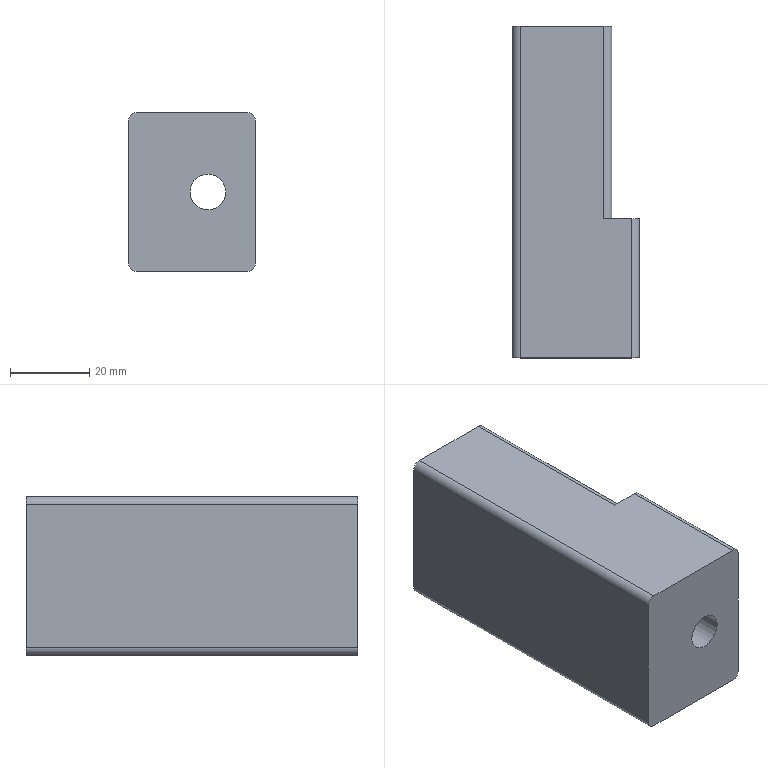Part | Mastercam | 1 solid | 26 faces | box 32 x 83.5 x 40 mm | volume 77489 mm3 | cylinder 15 | plane 11 | commonest cylinder face diameters 4 x8 9 x2 12 x2 16 x2 20 x1
STEP:
#1=CARTESIAN_POINT('',(0.,0.,0.));
#2=DIRECTION('',(0.,0.,1.));
#3=DIRECTION('',(1.,0.,0.));
#4=AXIS2_PLACEMENT_3D('',#1,#2,#3);
#5=CARTESIAN_POINT('',(12.,0.,18.));
#6=VERTEX_POINT('',#5);
#7=CARTESIAN_POINT('',(12.,0.,-18.));
#8=VERTEX_POINT('',#7);
#9=CARTESIAN_POINT('',(12.,0.,18.));
#10=DIRECTION('',(0.,0.,-1.));
#11=VECTOR('',#10,1.);
#12=LINE('',#9,#11);
#13=EDGE_CURVE('',#6,#8,#12,.T.);
#14=ORIENTED_EDGE('',*,*,#13,.F.);
#15=CARTESIAN_POINT('',(10.,0.,20.));
#16=VERTEX_POINT('',#15);
#17=CARTESIAN_POINT('',(10.,0.,18.));
#18=DIRECTION('',(0.,-1.,0.));
#19=DIRECTION('',(1.,0.,0.));
#20=AXIS2_PLACEMENT_3D('',#17,#18,#19);
#21=CIRCLE('',#20,2.);
#22=EDGE_CURVE('',#6,#16,#21,.T.);
#23=ORIENTED_EDGE('',*,*,#22,.T.);
#24=CARTESIAN_POINT('',(-18.,0.,20.));
#25=VERTEX_POINT('',#24);
#26=CARTESIAN_POINT('',(-18.,0.,20.));
#27=DIRECTION('',(1.,0.,0.));
#28=VECTOR('',#27,1.);
#29=LINE('',#26,#28);
#30=EDGE_CURVE('',#25,#16,#29,.T.);
#31=ORIENTED_EDGE('',*,*,#30,.F.);
#32=CARTESIAN_POINT('',(-20.,0.,18.));
#33=VERTEX_POINT('',#32);
#34=CARTESIAN_POINT('',(-18.,0.,18.));
#35=DIRECTION('',(0.,-1.,0.));
#36=DIRECTION('',(0.,0.,1.));
#37=AXIS2_PLACEMENT_3D('',#34,#35,#36);
#38=CIRCLE('',#37,2.);
#39=EDGE_CURVE('',#25,#33,#38,.T.);
#40=ORIENTED_EDGE('',*,*,#39,.T.);
#41=CARTESIAN_POINT('',(-20.,0.,-18.));
#42=VERTEX_POINT('',#41);
#43=CARTESIAN_POINT('',(-20.,0.,-18.));
#44=DIRECTION('',(0.,0.,1.));
#45=VECTOR('',#44,1.);
#46=LINE('',#43,#45);
#47=EDGE_CURVE('',#42,#33,#46,.T.);
#48=ORIENTED_EDGE('',*,*,#47,.F.);
#49=CARTESIAN_POINT('',(-18.,0.,-20.));
#50=VERTEX_POINT('',#49);
#51=CARTESIAN_POINT('',(-18.,0.,-18.));
#52=DIRECTION('',(0.,-1.,0.));
#53=DIRECTION('',(-1.,0.,0.));
#54=AXIS2_PLACEMENT_3D('',#51,#52,#53);
#55=CIRCLE('',#54,2.);
#56=EDGE_CURVE('',#42,#50,#55,.T.);
#57=ORIENTED_EDGE('',*,*,#56,.T.);
#58=CARTESIAN_POINT('',(10.,0.,-20.));
#59=VERTEX_POINT('',#58);
#60=CARTESIAN_POINT('',(10.,0.,-20.));
#61=DIRECTION('',(-1.,0.,0.));
#62=VECTOR('',#61,1.);
#63=LINE('',#60,#62);
#64=EDGE_CURVE('',#59,#50,#63,.T.);
#65=ORIENTED_EDGE('',*,*,#64,.F.);
#66=CARTESIAN_POINT('',(10.,0.,-18.));
#67=DIRECTION('',(0.,-1.,0.));
#68=DIRECTION('',(0.,0.,-1.));
#69=AXIS2_PLACEMENT_3D('',#66,#67,#68);
#70=CIRCLE('',#69,2.);
#71=EDGE_CURVE('',#59,#8,#70,.T.);
#72=ORIENTED_EDGE('',*,*,#71,.T.);
#73=EDGE_LOOP('',(#14,#23,#31,#40,#48,#57,#65,#72));
#74=FACE_OUTER_BOUND('',#73,.T.);
#75=CARTESIAN_POINT('',(4.5,0.,0.));
#76=VERTEX_POINT('',#75);
#77=CARTESIAN_POINT('',(0.,0.,4.5));
#78=VERTEX_POINT('',#77);
#79=CARTESIAN_POINT('',(0.,0.,0.));
#80=DIRECTION('',(0.,-1.,0.));
#81=DIRECTION('',(0.,0.,1.));
#82=AXIS2_PLACEMENT_3D('',#79,#80,#81);
#83=CIRCLE('',#82,4.5);
#84=EDGE_CURVE('',#76,#78,#83,.T.);
#85=ORIENTED_EDGE('',*,*,#84,.F.);
#86=CARTESIAN_POINT('',(-4.5,0.,0.));
#87=VERTEX_POINT('',#86);
#88=CARTESIAN_POINT('',(0.,0.,0.));
#89=DIRECTION('',(0.,-1.,0.));
#90=DIRECTION('',(0.,0.,1.));
#91=AXIS2_PLACEMENT_3D('',#88,#89,#90);
#92=CIRCLE('',#91,4.5);
#93=EDGE_CURVE('',#87,#76,#92,.T.);
#94=ORIENTED_EDGE('',*,*,#93,.F.);
#95=CARTESIAN_POINT('',(0.,0.,0.));
#96=DIRECTION('',(0.,-1.,0.));
#97=DIRECTION('',(0.,0.,1.));
#98=AXIS2_PLACEMENT_3D('',#95,#96,#97);
#99=CIRCLE('',#98,4.5);
#100=EDGE_CURVE('',#78,#87,#99,.T.);
#101=ORIENTED_EDGE('',*,*,#100,.F.);
#102=EDGE_LOOP('',(#85,#94,#101));
#103=FACE_BOUND('',#102,.T.);
#104=CARTESIAN_POINT('',(0.,0.,0.));
#105=DIRECTION('',(0.,1.,0.));
#106=DIRECTION('',(1.,0.,0.));
#107=AXIS2_PLACEMENT_3D('',#104,#105,#106);
#108=PLANE('',#107);
#109=ADVANCED_FACE('',(#74,#103),#108,.F.);
#110=CARTESIAN_POINT('',(-4.5,30.,0.));
#111=VERTEX_POINT('',#110);
#112=CARTESIAN_POINT('',(-4.5,30.,0.));
#113=DIRECTION('',(0.,-1.,0.));
#114=VECTOR('',#113,1.);
#115=LINE('',#112,#114);
#116=EDGE_CURVE('',#111,#87,#115,.T.);
#117=ORIENTED_EDGE('',*,*,#116,.T.);
#118=ORIENTED_EDGE('',*,*,#93,.T.);
#119=CARTESIAN_POINT('',(4.5,30.,0.));
#120=VERTEX_POINT('',#119);
#121=CARTESIAN_POINT('',(4.5,30.,0.));
#122=DIRECTION('',(0.,-1.,0.));
#123=VECTOR('',#122,1.);
#124=LINE('',#121,#123);
#125=EDGE_CURVE('',#120,#76,#124,.T.);
#126=ORIENTED_EDGE('',*,*,#125,.F.);
#127=CARTESIAN_POINT('',(0.,30.,0.));
#128=DIRECTION('',(0.,-1.,0.));
#129=DIRECTION('',(0.,0.,1.));
#130=AXIS2_PLACEMENT_3D('',#127,#128,#129);
#131=CIRCLE('',#130,4.5);
#132=EDGE_CURVE('',#111,#120,#131,.T.);
#133=ORIENTED_EDGE('',*,*,#132,.F.);
#134=EDGE_LOOP('',(#117,#118,#126,#133));
#135=FACE_OUTER_BOUND('',#134,.T.);
#136=CARTESIAN_POINT('',(0.,36.75,0.));
#137=DIRECTION('',(0.,-1.,0.));
#138=DIRECTION('',(0.,0.,1.));
#139=AXIS2_PLACEMENT_3D('',#136,#137,#138);
#140=CYLINDRICAL_SURFACE('',#139,4.5);
#141=ADVANCED_FACE('',(#135),#140,.F.);
#142=CARTESIAN_POINT('',(6.,30.,0.));
#143=VERTEX_POINT('',#142);
#144=CARTESIAN_POINT('',(0.,30.,6.));
#145=VERTEX_POINT('',#144);
#146=CARTESIAN_POINT('',(0.,30.,0.));
#147=DIRECTION('',(0.,-1.,0.));
#148=DIRECTION('',(0.,0.,1.));
#149=AXIS2_PLACEMENT_3D('',#146,#147,#148);
#150=CIRCLE('',#149,6.);
#151=EDGE_CURVE('',#143,#145,#150,.T.);
#152=ORIENTED_EDGE('',*,*,#151,.F.);
#153=CARTESIAN_POINT('',(-6.,30.,0.));
#154=VERTEX_POINT('',#153);
#155=CARTESIAN_POINT('',(0.,30.,0.));
#156=DIRECTION('',(0.,-1.,0.));
#157=DIRECTION('',(0.,0.,1.));
#158=AXIS2_PLACEMENT_3D('',#155,#156,#157);
#159=CIRCLE('',#158,6.);
#160=EDGE_CURVE('',#154,#143,#159,.T.);
#161=ORIENTED_EDGE('',*,*,#160,.F.);
#162=CARTESIAN_POINT('',(0.,30.,0.));
#163=DIRECTION('',(0.,-1.,0.));
#164=DIRECTION('',(0.,0.,1.));
#165=AXIS2_PLACEMENT_3D('',#162,#163,#164);
#166=CIRCLE('',#165,6.);
#167=EDGE_CURVE('',#145,#154,#166,.T.);
#168=ORIENTED_EDGE('',*,*,#167,.F.);
#169=EDGE_LOOP('',(#152,#161,#168));
#170=FACE_OUTER_BOUND('',#169,.T.);
#171=CARTESIAN_POINT('',(0.,30.,4.5));
#172=VERTEX_POINT('',#171);
#173=CARTESIAN_POINT('',(0.,30.,0.));
#174=DIRECTION('',(0.,-1.,0.));
#175=DIRECTION('',(0.,0.,1.));
#176=AXIS2_PLACEMENT_3D('',#173,#174,#175);
#177=CIRCLE('',#176,4.5);
#178=EDGE_CURVE('',#172,#111,#177,.T.);
#179=ORIENTED_EDGE('',*,*,#178,.T.);
#180=ORIENTED_EDGE('',*,*,#132,.T.);
#181=CARTESIAN_POINT('',(0.,30.,0.));
#182=DIRECTION('',(0.,-1.,0.));
#183=DIRECTION('',(0.,0.,1.));
#184=AXIS2_PLACEMENT_3D('',#181,#182,#183);
#185=CIRCLE('',#184,4.5);
#186=EDGE_CURVE('',#120,#172,#185,.T.);
#187=ORIENTED_EDGE('',*,*,#186,.T.);
#188=EDGE_LOOP('',(#179,#180,#187));
#189=FACE_BOUND('',#188,.T.);
#190=CARTESIAN_POINT('',(0.,30.,0.));
#191=DIRECTION('',(0.,-1.,0.));
#192=DIRECTION('',(0.,0.,1.));
#193=AXIS2_PLACEMENT_3D('',#190,#191,#192);
#194=PLANE('',#193);
#195=ADVANCED_FACE('',(#170,#189),#194,.F.);
#196=CARTESIAN_POINT('',(-6.,28.,0.));
#197=VERTEX_POINT('',#196);
#198=CARTESIAN_POINT('',(-6.,30.,0.));
#199=DIRECTION('',(0.,-1.,0.));
#200=VECTOR('',#199,1.);
#201=LINE('',#198,#200);
#202=EDGE_CURVE('',#154,#197,#201,.T.);
#203=ORIENTED_EDGE('',*,*,#202,.F.);
#204=ORIENTED_EDGE('',*,*,#160,.T.);
#205=CARTESIAN_POINT('',(6.,28.,0.));
#206=VERTEX_POINT('',#205);
#207=CARTESIAN_POINT('',(6.,30.,0.));
#208=DIRECTION('',(0.,-1.,0.));
#209=VECTOR('',#208,1.);
#210=LINE('',#207,#209);
#211=EDGE_CURVE('',#143,#206,#210,.T.);
#212=ORIENTED_EDGE('',*,*,#211,.T.);
#213=CARTESIAN_POINT('',(0.,28.,0.));
#214=DIRECTION('',(0.,-1.,0.));
#215=DIRECTION('',(0.,0.,1.));
#216=AXIS2_PLACEMENT_3D('',#213,#214,#215);
#217=CIRCLE('',#216,6.);
#218=EDGE_CURVE('',#197,#206,#217,.T.);
#219=ORIENTED_EDGE('',*,*,#218,.F.);
#220=EDGE_LOOP('',(#203,#204,#212,#219));
#221=FACE_OUTER_BOUND('',#220,.T.);
#222=CARTESIAN_POINT('',(0.,30.1,0.));
#223=DIRECTION('',(0.,-1.,0.));
#224=DIRECTION('',(0.,0.,1.));
#225=AXIS2_PLACEMENT_3D('',#222,#223,#224);
#226=CYLINDRICAL_SURFACE('',#225,6.);
#227=ADVANCED_FACE('',(#221),#226,.T.);
#228=CARTESIAN_POINT('',(8.,28.,0.));
#229=VERTEX_POINT('',#228);
#230=CARTESIAN_POINT('',(0.,28.,8.));
#231=VERTEX_POINT('',#230);
#232=CARTESIAN_POINT('',(0.,28.,0.));
#233=DIRECTION('',(0.,-1.,0.));
#234=DIRECTION('',(0.,0.,1.));
#235=AXIS2_PLACEMENT_3D('',#232,#233,#234);
#236=CIRCLE('',#235,8.);
#237=EDGE_CURVE('',#229,#231,#236,.T.);
#238=ORIENTED_EDGE('',*,*,#237,.F.);
#239=CARTESIAN_POINT('',(-8.,28.,0.));
#240=VERTEX_POINT('',#239);
#241=CARTESIAN_POINT('',(0.,28.,0.));
#242=DIRECTION('',(0.,-1.,0.));
#243=DIRECTION('',(0.,0.,1.));
#244=AXIS2_PLACEMENT_3D('',#241,#242,#243);
#245=CIRCLE('',#244,8.);
#246=EDGE_CURVE('',#240,#229,#245,.T.);
#247=ORIENTED_EDGE('',*,*,#246,.F.);
#248=CARTESIAN_POINT('',(0.,28.,0.));
#249=DIRECTION('',(0.,-1.,0.));
#250=DIRECTION('',(0.,0.,1.));
#251=AXIS2_PLACEMENT_3D('',#248,#249,#250);
#252=CIRCLE('',#251,8.);
#253=EDGE_CURVE('',#231,#240,#252,.T.);
#254=ORIENTED_EDGE('',*,*,#253,.F.);
#255=EDGE_LOOP('',(#238,#247,#254));
#256=FACE_OUTER_BOUND('',#255,.T.);
#257=CARTESIAN_POINT('',(0.,28.,6.));
#258=VERTEX_POINT('',#257);
#259=CARTESIAN_POINT('',(0.,28.,0.));
#260=DIRECTION('',(0.,-1.,0.));
#261=DIRECTION('',(0.,0.,1.));
#262=AXIS2_PLACEMENT_3D('',#259,#260,#261);
#263=CIRCLE('',#262,6.);
#264=EDGE_CURVE('',#258,#197,#263,.T.);
#265=ORIENTED_EDGE('',*,*,#264,.T.);
#266=ORIENTED_EDGE('',*,*,#218,.T.);
#267=CARTESIAN_POINT('',(0.,28.,0.));
#268=DIRECTION('',(0.,-1.,0.));
#269=DIRECTION('',(0.,0.,1.));
#270=AXIS2_PLACEMENT_3D('',#267,#268,#269);
#271=CIRCLE('',#270,6.);
#272=EDGE_CURVE('',#206,#258,#271,.T.);
#273=ORIENTED_EDGE('',*,*,#272,.T.);
#274=EDGE_LOOP('',(#265,#266,#273));
#275=FACE_BOUND('',#274,.T.);
#276=CARTESIAN_POINT('',(0.,28.,0.));
#277=DIRECTION('',(0.,-1.,0.));
#278=DIRECTION('',(0.,0.,1.));
#279=AXIS2_PLACEMENT_3D('',#276,#277,#278);
#280=PLANE('',#279);
#281=ADVANCED_FACE('',(#256,#275),#280,.F.);
#282=CARTESIAN_POINT('',(-8.,35.,0.));
#283=VERTEX_POINT('',#282);
#284=CARTESIAN_POINT('',(-8.,35.,0.));
#285=DIRECTION('',(0.,-1.,0.));
#286=VECTOR('',#285,1.);
#287=LINE('',#284,#286);
#288=EDGE_CURVE('',#283,#240,#287,.T.);
#289=ORIENTED_EDGE('',*,*,#288,.T.);
#290=ORIENTED_EDGE('',*,*,#246,.T.);
#291=CARTESIAN_POINT('',(8.,35.,0.));
#292=VERTEX_POINT('',#291);
#293=CARTESIAN_POINT('',(8.,35.,0.));
#294=DIRECTION('',(0.,-1.,0.));
#295=VECTOR('',#294,1.);
#296=LINE('',#293,#295);
#297=EDGE_CURVE('',#292,#229,#296,.T.);
#298=ORIENTED_EDGE('',*,*,#297,.F.);
#299=CARTESIAN_POINT('',(0.,35.,0.));
#300=DIRECTION('',(0.,-1.,0.));
#301=DIRECTION('',(0.,0.,1.));
#302=AXIS2_PLACEMENT_3D('',#299,#300,#301);
#303=CIRCLE('',#302,8.);
#304=EDGE_CURVE('',#283,#292,#303,.T.);
#305=ORIENTED_EDGE('',*,*,#304,.F.);
#306=EDGE_LOOP('',(#289,#290,#298,#305));
#307=FACE_OUTER_BOUND('',#306,.T.);
#308=CARTESIAN_POINT('',(0.,35.25,0.));
#309=DIRECTION('',(0.,-1.,0.));
#310=DIRECTION('',(0.,0.,1.));
#311=AXIS2_PLACEMENT_3D('',#308,#309,#310);
#312=CYLINDRICAL_SURFACE('',#311,8.);
#313=ADVANCED_FACE('',(#307),#312,.F.);
#314=CARTESIAN_POINT('',(5.,35.,-11.619));
#315=VERTEX_POINT('',#314);
#316=CARTESIAN_POINT('',(2.5,35.,-9.682));
#317=VERTEX_POINT('',#316);
#318=CARTESIAN_POINT('',(3.,35.,-11.619));
#319=DIRECTION('',(0.,-1.,0.));
#320=DIRECTION('',(1.,0.,0.));
#321=AXIS2_PLACEMENT_3D('',#318,#319,#320);
#322=CIRCLE('',#321,2.);
#323=EDGE_CURVE('',#315,#317,#322,.T.);
#324=ORIENTED_EDGE('',*,*,#323,.T.);
#325=CARTESIAN_POINT('',(2.5,35.,9.682));
#326=VERTEX_POINT('',#325);
#327=CARTESIAN_POINT('',(0.,35.,0.));
#328=DIRECTION('',(0.,1.,0.));
#329=DIRECTION('',(0.25,0.,-0.9682));
#330=AXIS2_PLACEMENT_3D('',#327,#328,#329);
#331=CIRCLE('',#330,10.);
#332=EDGE_CURVE('',#317,#326,#331,.T.);
#333=ORIENTED_EDGE('',*,*,#332,.T.);
#334=CARTESIAN_POINT('',(5.,35.,11.619));
#335=VERTEX_POINT('',#334);
#336=CARTESIAN_POINT('',(3.,35.,11.619));
#337=DIRECTION('',(0.,-1.,0.));
#338=DIRECTION('',(-0.25,0.,-0.9682));
#339=AXIS2_PLACEMENT_3D('',#336,#337,#338);
#340=CIRCLE('',#339,2.);
#341=EDGE_CURVE('',#326,#335,#340,.T.);
#342=ORIENTED_EDGE('',*,*,#341,.T.);
#343=CARTESIAN_POINT('',(5.,35.,18.));
#344=VERTEX_POINT('',#343);
#345=CARTESIAN_POINT('',(5.,35.,18.));
#346=DIRECTION('',(0.,0.,-1.));
#347=VECTOR('',#346,1.);
#348=LINE('',#345,#347);
#349=EDGE_CURVE('',#344,#335,#348,.T.);
#350=ORIENTED_EDGE('',*,*,#349,.F.);
#351=CARTESIAN_POINT('',(3.,35.,20.));
#352=VERTEX_POINT('',#351);
#353=CARTESIAN_POINT('',(3.,35.,18.));
#354=DIRECTION('',(0.,-1.,0.));
#355=DIRECTION('',(1.,0.,0.));
#356=AXIS2_PLACEMENT_3D('',#353,#354,#355);
#357=CIRCLE('',#356,2.);
#358=EDGE_CURVE('',#344,#352,#357,.T.);
#359=ORIENTED_EDGE('',*,*,#358,.T.);
#360=CARTESIAN_POINT('',(10.,35.,20.));
#361=VERTEX_POINT('',#360);
#362=CARTESIAN_POINT('',(10.,35.,20.));
#363=DIRECTION('',(-1.,0.,0.));
#364=VECTOR('',#363,1.);
#365=LINE('',#362,#364);
#366=EDGE_CURVE('',#361,#352,#365,.T.);
#367=ORIENTED_EDGE('',*,*,#366,.F.);
#368=CARTESIAN_POINT('',(12.,35.,18.));
#369=VERTEX_POINT('',#368);
#370=CARTESIAN_POINT('',(10.,35.,18.));
#371=DIRECTION('',(0.,1.,0.));
#372=DIRECTION('',(0.,0.,1.));
#373=AXIS2_PLACEMENT_3D('',#370,#371,#372);
#374=CIRCLE('',#373,2.);
#375=EDGE_CURVE('',#361,#369,#374,.T.);
#376=ORIENTED_EDGE('',*,*,#375,.T.);
#377=CARTESIAN_POINT('',(12.,35.,-18.));
#378=VERTEX_POINT('',#377);
#379=CARTESIAN_POINT('',(12.,35.,18.));
#380=DIRECTION('',(0.,0.,-1.));
#381=VECTOR('',#380,1.);
#382=LINE('',#379,#381);
#383=EDGE_CURVE('',#369,#378,#382,.T.);
#384=ORIENTED_EDGE('',*,*,#383,.T.);
#385=CARTESIAN_POINT('',(10.,35.,-20.));
#386=VERTEX_POINT('',#385);
#387=CARTESIAN_POINT('',(10.,35.,-18.));
#388=DIRECTION('',(0.,1.,0.));
#389=DIRECTION('',(1.,0.,0.));
#390=AXIS2_PLACEMENT_3D('',#387,#388,#389);
#391=CIRCLE('',#390,2.);
#392=EDGE_CURVE('',#378,#386,#391,.T.);
#393=ORIENTED_EDGE('',*,*,#392,.T.);
#394=CARTESIAN_POINT('',(3.,35.,-20.));
#395=VERTEX_POINT('',#394);
#396=CARTESIAN_POINT('',(3.,35.,-20.));
#397=DIRECTION('',(1.,0.,0.));
#398=VECTOR('',#397,1.);
#399=LINE('',#396,#398);
#400=EDGE_CURVE('',#395,#386,#399,.T.);
#401=ORIENTED_EDGE('',*,*,#400,.F.);
#402=CARTESIAN_POINT('',(5.,35.,-18.));
#403=VERTEX_POINT('',#402);
#404=CARTESIAN_POINT('',(3.,35.,-18.));
#405=DIRECTION('',(0.,-1.,0.));
#406=DIRECTION('',(0.,0.,-1.));
#407=AXIS2_PLACEMENT_3D('',#404,#405,#406);
#408=CIRCLE('',#407,2.);
#409=EDGE_CURVE('',#395,#403,#408,.T.);
#410=ORIENTED_EDGE('',*,*,#409,.T.);
#411=CARTESIAN_POINT('',(5.,35.,-11.619));
#412=DIRECTION('',(0.,0.,-1.));
#413=VECTOR('',#412,1.);
#414=LINE('',#411,#413);
#415=EDGE_CURVE('',#315,#403,#414,.T.);
#416=ORIENTED_EDGE('',*,*,#415,.F.);
#417=EDGE_LOOP('',(#324,#333,#342,#350,#359,#367,#376,#384,#393,#401,#410,#416));
#418=FACE_OUTER_BOUND('',#417,.T.);
#419=CARTESIAN_POINT('',(0.,35.,8.));
#420=VERTEX_POINT('',#419);
#421=CARTESIAN_POINT('',(0.,35.,0.));
#422=DIRECTION('',(0.,-1.,0.));
#423=DIRECTION('',(0.,0.,1.));
#424=AXIS2_PLACEMENT_3D('',#421,#422,#423);
#425=CIRCLE('',#424,8.);
#426=EDGE_CURVE('',#420,#283,#425,.T.);
#427=ORIENTED_EDGE('',*,*,#426,.T.);
#428=ORIENTED_EDGE('',*,*,#304,.T.);
#429=CARTESIAN_POINT('',(0.,35.,0.));
#430=DIRECTION('',(0.,-1.,0.));
#431=DIRECTION('',(0.,0.,1.));
#432=AXIS2_PLACEMENT_3D('',#429,#430,#431);
#433=CIRCLE('',#432,8.);
#434=EDGE_CURVE('',#292,#420,#433,.T.);
#435=ORIENTED_EDGE('',*,*,#434,.T.);
#436=EDGE_LOOP('',(#427,#428,#435));
#437=FACE_BOUND('',#436,.T.);
#438=CARTESIAN_POINT('',(0.,35.,0.));
#439=DIRECTION('',(0.,-1.,0.));
#440=DIRECTION('',(0.,0.,1.));
#441=AXIS2_PLACEMENT_3D('',#438,#439,#440);
#442=PLANE('',#441);
#443=ADVANCED_FACE('',(#418,#437),#442,.F.);
#444=CARTESIAN_POINT('',(5.,83.5,-11.619));
#445=VERTEX_POINT('',#444);
#446=CARTESIAN_POINT('',(5.,83.5,-18.));
#447=VERTEX_POINT('',#446);
#448=CARTESIAN_POINT('',(5.,83.5,-11.619));
#449=DIRECTION('',(0.,0.,-1.));
#450=VECTOR('',#449,1.);
#451=LINE('',#448,#450);
#452=EDGE_CURVE('',#445,#447,#451,.T.);
#453=ORIENTED_EDGE('',*,*,#452,.F.);
#454=CARTESIAN_POINT('',(5.,35.,-11.619));
#455=DIRECTION('',(0.,1.,0.));
#456=VECTOR('',#455,1.);
#457=LINE('',#454,#456);
#458=EDGE_CURVE('',#315,#445,#457,.T.);
#459=ORIENTED_EDGE('',*,*,#458,.F.);
#460=ORIENTED_EDGE('',*,*,#415,.T.);
#461=CARTESIAN_POINT('',(5.,83.5,-18.));
#462=DIRECTION('',(0.,-1.,0.));
#463=VECTOR('',#462,1.);
#464=LINE('',#461,#463);
#465=EDGE_CURVE('',#447,#403,#464,.T.);
#466=ORIENTED_EDGE('',*,*,#465,.F.);
#467=EDGE_LOOP('',(#453,#459,#460,#466));
#468=FACE_OUTER_BOUND('',#467,.T.);
#469=CARTESIAN_POINT('',(5.,0.,0.));
#470=DIRECTION('',(1.,0.,0.));
#471=DIRECTION('',(0.,0.,-1.));
#472=AXIS2_PLACEMENT_3D('',#469,#470,#471);
#473=PLANE('',#472);
#474=ADVANCED_FACE('',(#468),#473,.T.);
#475=ORIENTED_EDGE('',*,*,#409,.F.);
#476=CARTESIAN_POINT('',(3.,83.5,-20.));
#477=VERTEX_POINT('',#476);
#478=CARTESIAN_POINT('',(3.,83.5,-20.));
#479=DIRECTION('',(0.,-1.,0.));
#480=VECTOR('',#479,1.);
#481=LINE('',#478,#480);
#482=EDGE_CURVE('',#477,#395,#481,.T.);
#483=ORIENTED_EDGE('',*,*,#482,.F.);
#484=CARTESIAN_POINT('',(3.,83.5,-18.));
#485=DIRECTION('',(0.,1.,0.));
#486=DIRECTION('',(1.,0.,0.));
#487=AXIS2_PLACEMENT_3D('',#484,#485,#486);
#488=CIRCLE('',#487,2.);
#489=EDGE_CURVE('',#447,#477,#488,.T.);
#490=ORIENTED_EDGE('',*,*,#489,.F.);
#491=ORIENTED_EDGE('',*,*,#465,.T.);
#492=EDGE_LOOP('',(#475,#483,#490,#491));
#493=FACE_OUTER_BOUND('',#492,.T.);
#494=CARTESIAN_POINT('',(3.,192.351,-18.));
#495=DIRECTION('',(0.,-1.,0.));
#496=DIRECTION('',(-0.7071,0.,0.7071));
#497=AXIS2_PLACEMENT_3D('',#494,#495,#496);
#498=CYLINDRICAL_SURFACE('',#497,2.);
#499=ADVANCED_FACE('',(#493),#498,.T.);
#500=CARTESIAN_POINT('',(5.,83.5,18.));
#501=VERTEX_POINT('',#500);
#502=CARTESIAN_POINT('',(5.,83.5,11.619));
#503=VERTEX_POINT('',#502);
#504=CARTESIAN_POINT('',(5.,83.5,18.));
#505=DIRECTION('',(0.,0.,-1.));
#506=VECTOR('',#505,1.);
#507=LINE('',#504,#506);
#508=EDGE_CURVE('',#501,#503,#507,.T.);
#509=ORIENTED_EDGE('',*,*,#508,.T.);
#510=CARTESIAN_POINT('',(2.5,83.5,9.682));
#511=VERTEX_POINT('',#510);
#512=CARTESIAN_POINT('',(3.,83.5,11.619));
#513=DIRECTION('',(0.,1.,0.));
#514=DIRECTION('',(1.,0.,0.));
#515=AXIS2_PLACEMENT_3D('',#512,#513,#514);
#516=CIRCLE('',#515,2.);
#517=EDGE_CURVE('',#503,#511,#516,.T.);
#518=ORIENTED_EDGE('',*,*,#517,.T.);
#519=CARTESIAN_POINT('',(2.5,83.5,-9.682));
#520=VERTEX_POINT('',#519);
#521=CARTESIAN_POINT('',(0.,83.5,0.));
#522=DIRECTION('',(0.,-1.,0.));
#523=DIRECTION('',(0.25,0.,0.9682));
#524=AXIS2_PLACEMENT_3D('',#521,#522,#523);
#525=CIRCLE('',#524,10.);
#526=EDGE_CURVE('',#511,#520,#525,.T.);
#527=ORIENTED_EDGE('',*,*,#526,.T.);
#528=CARTESIAN_POINT('',(3.,83.5,-11.619));
#529=DIRECTION('',(0.,1.,0.));
#530=DIRECTION('',(-0.25,0.,0.9682));
#531=AXIS2_PLACEMENT_3D('',#528,#529,#530);
#532=CIRCLE('',#531,2.);
#533=EDGE_CURVE('',#520,#445,#532,.T.);
#534=ORIENTED_EDGE('',*,*,#533,.T.);
#535=ORIENTED_EDGE('',*,*,#452,.T.);
#536=ORIENTED_EDGE('',*,*,#489,.T.);
#537=CARTESIAN_POINT('',(-18.,83.5,-20.));
#538=VERTEX_POINT('',#537);
#539=CARTESIAN_POINT('',(3.,83.5,-20.));
#540=DIRECTION('',(-1.,0.,0.));
#541=VECTOR('',#540,1.);
#542=LINE('',#539,#541);
#543=EDGE_CURVE('',#477,#538,#542,.T.);
#544=ORIENTED_EDGE('',*,*,#543,.T.);
#545=CARTESIAN_POINT('',(-20.,83.5,-18.));
#546=VERTEX_POINT('',#545);
#547=CARTESIAN_POINT('',(-18.,83.5,-18.));
#548=DIRECTION('',(0.,1.,0.));
#549=DIRECTION('',(0.,0.,-1.));
#550=AXIS2_PLACEMENT_3D('',#547,#548,#549);
#551=CIRCLE('',#550,2.);
#552=EDGE_CURVE('',#538,#546,#551,.T.);
#553=ORIENTED_EDGE('',*,*,#552,.T.);
#554=CARTESIAN_POINT('',(-20.,83.5,18.));
#555=VERTEX_POINT('',#554);
#556=CARTESIAN_POINT('',(-20.,83.5,-18.));
#557=DIRECTION('',(0.,0.,1.));
#558=VECTOR('',#557,1.);
#559=LINE('',#556,#558);
#560=EDGE_CURVE('',#546,#555,#559,.T.);
#561=ORIENTED_EDGE('',*,*,#560,.T.);
#562=CARTESIAN_POINT('',(-18.,83.5,20.));
#563=VERTEX_POINT('',#562);
#564=CARTESIAN_POINT('',(-18.,83.5,18.));
#565=DIRECTION('',(0.,1.,0.));
#566=DIRECTION('',(-1.,0.,0.));
#567=AXIS2_PLACEMENT_3D('',#564,#565,#566);
#568=CIRCLE('',#567,2.);
#569=EDGE_CURVE('',#555,#563,#568,.T.);
#570=ORIENTED_EDGE('',*,*,#569,.T.);
#571=CARTESIAN_POINT('',(3.,83.5,20.));
#572=VERTEX_POINT('',#571);
#573=CARTESIAN_POINT('',(-18.,83.5,20.));
#574=DIRECTION('',(1.,0.,0.));
#575=VECTOR('',#574,1.);
#576=LINE('',#573,#575);
#577=EDGE_CURVE('',#563,#572,#576,.T.);
#578=ORIENTED_EDGE('',*,*,#577,.T.);
#579=CARTESIAN_POINT('',(3.,83.5,18.));
#580=DIRECTION('',(0.,1.,0.));
#581=DIRECTION('',(0.,0.,1.));
#582=AXIS2_PLACEMENT_3D('',#579,#580,#581);
#583=CIRCLE('',#582,2.);
#584=EDGE_CURVE('',#572,#501,#583,.T.);
#585=ORIENTED_EDGE('',*,*,#584,.T.);
#586=EDGE_LOOP('',(#509,#518,#527,#534,#535,#536,#544,#553,#561,#570,#578,#585));
#587=FACE_OUTER_BOUND('',#586,.T.);
#588=CARTESIAN_POINT('',(0.,83.5,0.));
#589=DIRECTION('',(0.,1.,0.));
#590=DIRECTION('',(1.,0.,0.));
#591=AXIS2_PLACEMENT_3D('',#588,#589,#590);
#592=PLANE('',#591);
#593=ADVANCED_FACE('',(#587),#592,.T.);
#594=CARTESIAN_POINT('',(3.,35.,20.));
#595=DIRECTION('',(0.,1.,0.));
#596=VECTOR('',#595,1.);
#597=LINE('',#594,#596);
#598=EDGE_CURVE('',#352,#572,#597,.T.);
#599=ORIENTED_EDGE('',*,*,#598,.F.);
#600=ORIENTED_EDGE('',*,*,#358,.F.);
#601=CARTESIAN_POINT('',(5.,35.,18.));
#602=DIRECTION('',(0.,1.,0.));
#603=VECTOR('',#602,1.);
#604=LINE('',#601,#603);
#605=EDGE_CURVE('',#344,#501,#604,.T.);
#606=ORIENTED_EDGE('',*,*,#605,.T.);
#607=ORIENTED_EDGE('',*,*,#584,.F.);
#608=EDGE_LOOP('',(#599,#600,#606,#607));
#609=FACE_OUTER_BOUND('',#608,.T.);
#610=CARTESIAN_POINT('',(3.,-108.851,18.));
#611=DIRECTION('',(0.,1.,0.));
#612=DIRECTION('',(-0.7071,0.,-0.7071));
#613=AXIS2_PLACEMENT_3D('',#610,#611,#612);
#614=CYLINDRICAL_SURFACE('',#613,2.);
#615=ADVANCED_FACE('',(#609),#614,.T.);
#616=ORIENTED_EDGE('',*,*,#349,.T.);
#617=CARTESIAN_POINT('',(5.,83.5,11.619));
#618=DIRECTION('',(0.,-1.,0.));
#619=VECTOR('',#618,1.);
#620=LINE('',#617,#619);
#621=EDGE_CURVE('',#503,#335,#620,.T.);
#622=ORIENTED_EDGE('',*,*,#621,.F.);
#623=ORIENTED_EDGE('',*,*,#508,.F.);
#624=ORIENTED_EDGE('',*,*,#605,.F.);
#625=EDGE_LOOP('',(#616,#622,#623,#624));
#626=FACE_OUTER_BOUND('',#625,.T.);
#627=CARTESIAN_POINT('',(5.,0.,0.));
#628=DIRECTION('',(1.,0.,0.));
#629=DIRECTION('',(0.,0.,-1.));
#630=AXIS2_PLACEMENT_3D('',#627,#628,#629);
#631=PLANE('',#630);
#632=ADVANCED_FACE('',(#626),#631,.T.);
#633=ORIENTED_EDGE('',*,*,#341,.F.);
#634=CARTESIAN_POINT('',(2.5,83.5,9.682));
#635=DIRECTION('',(0.,-1.,0.));
#636=VECTOR('',#635,1.);
#637=LINE('',#634,#636);
#638=EDGE_CURVE('',#511,#326,#637,.T.);
#639=ORIENTED_EDGE('',*,*,#638,.F.);
#640=ORIENTED_EDGE('',*,*,#517,.F.);
#641=ORIENTED_EDGE('',*,*,#621,.T.);
#642=EDGE_LOOP('',(#633,#639,#640,#641));
#643=FACE_OUTER_BOUND('',#642,.T.);
#644=CARTESIAN_POINT('',(3.,192.351,11.619));
#645=DIRECTION('',(0.,-1.,0.));
#646=DIRECTION('',(-0.6124,0.,0.7906));
#647=AXIS2_PLACEMENT_3D('',#644,#645,#646);
#648=CYLINDRICAL_SURFACE('',#647,2.);
#649=ADVANCED_FACE('',(#643),#648,.T.);
#650=ORIENTED_EDGE('',*,*,#526,.F.);
#651=ORIENTED_EDGE('',*,*,#638,.T.);
#652=ORIENTED_EDGE('',*,*,#332,.F.);
#653=CARTESIAN_POINT('',(2.5,35.,-9.682));
#654=DIRECTION('',(0.,1.,0.));
#655=VECTOR('',#654,1.);
#656=LINE('',#653,#655);
#657=EDGE_CURVE('',#317,#520,#656,.T.);
#658=ORIENTED_EDGE('',*,*,#657,.T.);
#659=EDGE_LOOP('',(#650,#651,#652,#658));
#660=FACE_OUTER_BOUND('',#659,.T.);
#661=CARTESIAN_POINT('',(0.,85.925,0.));
#662=DIRECTION('',(0.,-1.,0.));
#663=DIRECTION('',(1.,0.,0.));
#664=AXIS2_PLACEMENT_3D('',#661,#662,#663);
#665=CYLINDRICAL_SURFACE('',#664,10.);
#666=ADVANCED_FACE('',(#660),#665,.F.);
#667=ORIENTED_EDGE('',*,*,#657,.F.);
#668=ORIENTED_EDGE('',*,*,#323,.F.);
#669=ORIENTED_EDGE('',*,*,#458,.T.);
#670=ORIENTED_EDGE('',*,*,#533,.F.);
#671=EDGE_LOOP('',(#667,#668,#669,#670));
#672=FACE_OUTER_BOUND('',#671,.T.);
#673=CARTESIAN_POINT('',(3.,-108.851,-11.619));
#674=DIRECTION('',(0.,1.,0.));
#675=DIRECTION('',(-0.6124,0.,-0.7906));
#676=AXIS2_PLACEMENT_3D('',#673,#674,#675);
#677=CYLINDRICAL_SURFACE('',#676,2.);
#678=ADVANCED_FACE('',(#672),#677,.T.);
#679=ORIENTED_EDGE('',*,*,#577,.F.);
#680=CARTESIAN_POINT('',(-18.,83.5,20.));
#681=DIRECTION('',(0.,-1.,0.));
#682=VECTOR('',#681,1.);
#683=LINE('',#680,#682);
#684=EDGE_CURVE('',#563,#25,#683,.T.);
#685=ORIENTED_EDGE('',*,*,#684,.T.);
#686=ORIENTED_EDGE('',*,*,#30,.T.);
#687=CARTESIAN_POINT('',(10.,35.,20.));
#688=DIRECTION('',(0.,-1.,0.));
#689=VECTOR('',#688,1.);
#690=LINE('',#687,#689);
#691=EDGE_CURVE('',#361,#16,#690,.T.);
#692=ORIENTED_EDGE('',*,*,#691,.F.);
#693=ORIENTED_EDGE('',*,*,#366,.T.);
#694=ORIENTED_EDGE('',*,*,#598,.T.);
#695=EDGE_LOOP('',(#679,#685,#686,#692,#693,#694));
#696=FACE_OUTER_BOUND('',#695,.T.);
#697=CARTESIAN_POINT('',(-20.,0.,20.));
#698=DIRECTION('',(0.,0.,1.));
#699=DIRECTION('',(1.,0.,0.));
#700=AXIS2_PLACEMENT_3D('',#697,#698,#699);
#701=PLANE('',#700);
#702=ADVANCED_FACE('',(#696),#701,.T.);
#703=CARTESIAN_POINT('',(12.,35.,18.));
#704=DIRECTION('',(0.,-1.,0.));
#705=VECTOR('',#704,1.);
#706=LINE('',#703,#705);
#707=EDGE_CURVE('',#369,#6,#706,.T.);
#708=ORIENTED_EDGE('',*,*,#707,.F.);
#709=ORIENTED_EDGE('',*,*,#375,.F.);
#710=ORIENTED_EDGE('',*,*,#691,.T.);
#711=ORIENTED_EDGE('',*,*,#22,.F.);
#712=EDGE_LOOP('',(#708,#709,#710,#711));
#713=FACE_OUTER_BOUND('',#712,.T.);
#714=CARTESIAN_POINT('',(10.,192.351,18.));
#715=DIRECTION('',(0.,-1.,0.));
#716=DIRECTION('',(-0.7071,0.,-0.7071));
#717=AXIS2_PLACEMENT_3D('',#714,#715,#716);
#718=CYLINDRICAL_SURFACE('',#717,2.);
#719=ADVANCED_FACE('',(#713),#718,.T.);
#720=ORIENTED_EDGE('',*,*,#383,.F.);
#721=ORIENTED_EDGE('',*,*,#707,.T.);
#722=ORIENTED_EDGE('',*,*,#13,.T.);
#723=CARTESIAN_POINT('',(12.,35.,-18.));
#724=DIRECTION('',(0.,-1.,0.));
#725=VECTOR('',#724,1.);
#726=LINE('',#723,#725);
#727=EDGE_CURVE('',#378,#8,#726,.T.);
#728=ORIENTED_EDGE('',*,*,#727,.F.);
#729=EDGE_LOOP('',(#720,#721,#722,#728));
#730=FACE_OUTER_BOUND('',#729,.T.);
#731=CARTESIAN_POINT('',(12.,0.,20.));
#732=DIRECTION('',(1.,0.,0.));
#733=DIRECTION('',(0.,0.,-1.));
#734=AXIS2_PLACEMENT_3D('',#731,#732,#733);
#735=PLANE('',#734);
#736=ADVANCED_FACE('',(#730),#735,.T.);
#737=CARTESIAN_POINT('',(10.,35.,-20.));
#738=DIRECTION('',(0.,-1.,0.));
#739=VECTOR('',#738,1.);
#740=LINE('',#737,#739);
#741=EDGE_CURVE('',#386,#59,#740,.T.);
#742=ORIENTED_EDGE('',*,*,#741,.F.);
#743=ORIENTED_EDGE('',*,*,#392,.F.);
#744=ORIENTED_EDGE('',*,*,#727,.T.);
#745=ORIENTED_EDGE('',*,*,#71,.F.);
#746=EDGE_LOOP('',(#742,#743,#744,#745));
#747=FACE_OUTER_BOUND('',#746,.T.);
#748=CARTESIAN_POINT('',(10.,192.351,-18.));
#749=DIRECTION('',(0.,-1.,0.));
#750=DIRECTION('',(-0.7071,0.,0.7071));
#751=AXIS2_PLACEMENT_3D('',#748,#749,#750);
#752=CYLINDRICAL_SURFACE('',#751,2.);
#753=ADVANCED_FACE('',(#747),#752,.T.);
#754=ORIENTED_EDGE('',*,*,#400,.T.);
#755=ORIENTED_EDGE('',*,*,#741,.T.);
#756=ORIENTED_EDGE('',*,*,#64,.T.);
#757=CARTESIAN_POINT('',(-18.,83.5,-20.));
#758=DIRECTION('',(0.,-1.,0.));
#759=VECTOR('',#758,1.);
#760=LINE('',#757,#759);
#761=EDGE_CURVE('',#538,#50,#760,.T.);
#762=ORIENTED_EDGE('',*,*,#761,.F.);
#763=ORIENTED_EDGE('',*,*,#543,.F.);
#764=ORIENTED_EDGE('',*,*,#482,.T.);
#765=EDGE_LOOP('',(#754,#755,#756,#762,#763,#764));
#766=FACE_OUTER_BOUND('',#765,.T.);
#767=CARTESIAN_POINT('',(12.,0.,-20.));
#768=DIRECTION('',(0.,0.,-1.));
#769=DIRECTION('',(-1.,0.,0.));
#770=AXIS2_PLACEMENT_3D('',#767,#768,#769);
#771=PLANE('',#770);
#772=ADVANCED_FACE('',(#766),#771,.T.);
#773=CARTESIAN_POINT('',(-20.,83.5,-18.));
#774=DIRECTION('',(0.,-1.,0.));
#775=VECTOR('',#774,1.);
#776=LINE('',#773,#775);
#777=EDGE_CURVE('',#546,#42,#776,.T.);
#778=ORIENTED_EDGE('',*,*,#777,.F.);
#779=ORIENTED_EDGE('',*,*,#552,.F.);
#780=ORIENTED_EDGE('',*,*,#761,.T.);
#781=ORIENTED_EDGE('',*,*,#56,.F.);
#782=EDGE_LOOP('',(#778,#779,#780,#781));
#783=FACE_OUTER_BOUND('',#782,.T.);
#784=CARTESIAN_POINT('',(-18.,192.351,-18.));
#785=DIRECTION('',(0.,-1.,0.));
#786=DIRECTION('',(0.7071,0.,0.7071));
#787=AXIS2_PLACEMENT_3D('',#784,#785,#786);
#788=CYLINDRICAL_SURFACE('',#787,2.);
#789=ADVANCED_FACE('',(#783),#788,.T.);
#790=ORIENTED_EDGE('',*,*,#560,.F.);
#791=ORIENTED_EDGE('',*,*,#777,.T.);
#792=ORIENTED_EDGE('',*,*,#47,.T.);
#793=CARTESIAN_POINT('',(-20.,83.5,18.));
#794=DIRECTION('',(0.,-1.,0.));
#795=VECTOR('',#794,1.);
#796=LINE('',#793,#795);
#797=EDGE_CURVE('',#555,#33,#796,.T.);
#798=ORIENTED_EDGE('',*,*,#797,.F.);
#799=EDGE_LOOP('',(#790,#791,#792,#798));
#800=FACE_OUTER_BOUND('',#799,.T.);
#801=CARTESIAN_POINT('',(-20.,0.,-20.));
#802=DIRECTION('',(-1.,0.,0.));
#803=DIRECTION('',(0.,0.,1.));
#804=AXIS2_PLACEMENT_3D('',#801,#802,#803);
#805=PLANE('',#804);
#806=ADVANCED_FACE('',(#800),#805,.T.);
#807=ORIENTED_EDGE('',*,*,#684,.F.);
#808=ORIENTED_EDGE('',*,*,#569,.F.);
#809=ORIENTED_EDGE('',*,*,#797,.T.);
#810=ORIENTED_EDGE('',*,*,#39,.F.);
#811=EDGE_LOOP('',(#807,#808,#809,#810));
#812=FACE_OUTER_BOUND('',#811,.T.);
#813=CARTESIAN_POINT('',(-18.,192.351,18.));
#814=DIRECTION('',(0.,-1.,0.));
#815=DIRECTION('',(0.7071,0.,-0.7071));
#816=AXIS2_PLACEMENT_3D('',#813,#814,#815);
#817=CYLINDRICAL_SURFACE('',#816,2.);
#818=ADVANCED_FACE('',(#812),#817,.T.);
#819=ORIENTED_EDGE('',*,*,#116,.F.);
#820=ORIENTED_EDGE('',*,*,#178,.F.);
#821=ORIENTED_EDGE('',*,*,#186,.F.);
#822=ORIENTED_EDGE('',*,*,#125,.T.);
#823=ORIENTED_EDGE('',*,*,#84,.T.);
#824=ORIENTED_EDGE('',*,*,#100,.T.);
#825=EDGE_LOOP('',(#819,#820,#821,#822,#823,#824));
#826=FACE_OUTER_BOUND('',#825,.T.);
#827=CARTESIAN_POINT('',(0.,36.75,0.));
#828=DIRECTION('',(0.,-1.,0.));
#829=DIRECTION('',(0.,0.,-1.));
#830=AXIS2_PLACEMENT_3D('',#827,#828,#829);
#831=CYLINDRICAL_SURFACE('',#830,4.5);
#832=ADVANCED_FACE('',(#826),#831,.F.);
#833=ORIENTED_EDGE('',*,*,#202,.T.);
#834=ORIENTED_EDGE('',*,*,#264,.F.);
#835=ORIENTED_EDGE('',*,*,#272,.F.);
#836=ORIENTED_EDGE('',*,*,#211,.F.);
#837=ORIENTED_EDGE('',*,*,#151,.T.);
#838=ORIENTED_EDGE('',*,*,#167,.T.);
#839=EDGE_LOOP('',(#833,#834,#835,#836,#837,#838));
#840=FACE_OUTER_BOUND('',#839,.T.);
#841=CARTESIAN_POINT('',(0.,30.1,0.));
#842=DIRECTION('',(0.,-1.,0.));
#843=DIRECTION('',(0.,0.,-1.));
#844=AXIS2_PLACEMENT_3D('',#841,#842,#843);
#845=CYLINDRICAL_SURFACE('',#844,6.);
#846=ADVANCED_FACE('',(#840),#845,.T.);
#847=ORIENTED_EDGE('',*,*,#288,.F.);
#848=ORIENTED_EDGE('',*,*,#426,.F.);
#849=ORIENTED_EDGE('',*,*,#434,.F.);
#850=ORIENTED_EDGE('',*,*,#297,.T.);
#851=ORIENTED_EDGE('',*,*,#237,.T.);
#852=ORIENTED_EDGE('',*,*,#253,.T.);
#853=EDGE_LOOP('',(#847,#848,#849,#850,#851,#852));
#854=FACE_OUTER_BOUND('',#853,.T.);
#855=CARTESIAN_POINT('',(0.,35.25,0.));
#856=DIRECTION('',(0.,-1.,0.));
#857=DIRECTION('',(0.,0.,-1.));
#858=AXIS2_PLACEMENT_3D('',#855,#856,#857);
#859=CYLINDRICAL_SURFACE('',#858,8.);
#860=ADVANCED_FACE('',(#854),#859,.F.);
#861=CLOSED_SHELL('',(#109,#141,#195,#227,#281,#313,#443,#474,#499,#593,#615,#632,#649,#666,#678,#702,#719,#736,#753,#772,#789,#806,#818,#832,#846,#860));
#862=MANIFOLD_SOLID_BREP('',#861);
#863=(LENGTH_UNIT()NAMED_UNIT(*)SI_UNIT(.MILLI.,.METRE.));
#864=UNCERTAINTY_MEASURE_WITH_UNIT(LENGTH_MEASURE(0.005),#863,'','');
#865=(NAMED_UNIT(*)PLANE_ANGLE_UNIT()SI_UNIT($,.RADIAN.));
#866=(GEOMETRIC_REPRESENTATION_CONTEXT(3)GLOBAL_UNCERTAINTY_ASSIGNED_CONTEXT((#864))GLOBAL_UNIT_ASSIGNED_CONTEXT((#863,#865))REPRESENTATION_CONTEXT('',''));
#867=ADVANCED_BREP_SHAPE_REPRESENTATION('',(#4,#862),#866);